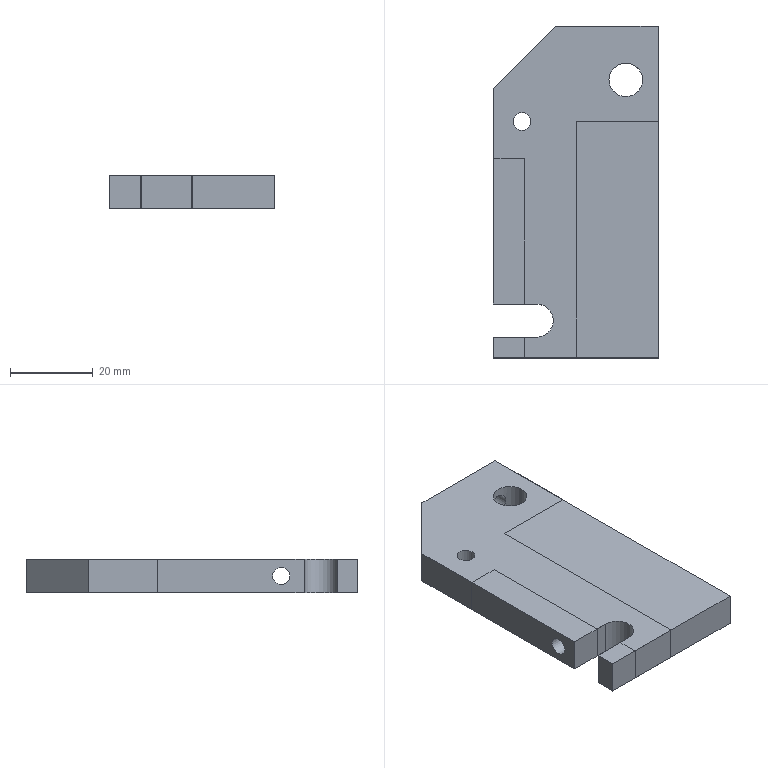NC program | NX | posted with a generic post | part box 40 x 80 x 8 mm
Lines 1 to 594 of 5028:
N10 G17 G21 G94 G90
(FLOOR_FACING_1 , TOOL : D63面刀)
N12 T10 M6
N14 G53
N16 G17 G0 G90 X74.501 Y-4.25 B0. C0. S1600 M3
N18 G43 Z20. H10
N20 Z3.
N22 G94 G1 Z0. F600.
N24 X71.501
N26 X-71.499
N28 X-74.499
N30 Z3.
N32 G0 Z20.
N34 M5
(动态粗 , TOOL : D10-30-D10-75-3T-ROUGH)
N36 T01 M6
N38 G53
N40 G17 G0 G90 X0.648 Y-30.538 B0. C0. S3500 M3
N42 G43 Z20. H1
N44 Z-9.5
N46 G94 G1 X0.649 Y-30.513 Z-9.656 F1500.
N48 X0.651 Y-30.488 Z-9.718
N50 X0.653 Y-30.463 Z-9.763
N52 X0.654 Y-30.438 Z-9.8
N54 X0.656 Y-30.413 Z-9.831
N56 X0.658 Y-30.388 Z-9.857
N58 X0.659 Y-30.363 Z-9.88
N60 X0.661 Y-30.338 Z-9.9
N62 X0.663 Y-30.313 Z-9.918
N64 X0.664 Y-30.288 Z-9.933
N66 X0.666 Y-30.263 Z-9.947
N68 X0.668 Y-30.238 Z-9.958
N70 X0.67 Y-30.213 Z-9.968
N72 X0.671 Y-30.188 Z-9.977
N74 X0.673 Y-30.163 Z-9.984
N76 X0.675 Y-30.139 Z-9.99
N78 X0.676 Y-30.114 Z-9.994
N80 X0.678 Y-30.089 Z-9.997
N82 X0.68 Y-30.064 Z-9.999
N84 X0.681 Y-30.039 Z-10.
N86 X0.78 Y-28.563
N88 G3 X0.004 Y-27.512 R1.01
N90 X-3.302 Y-27.236 R17.164
N92 X-10.4 Y-27.2 R609.799
N94 G1 X-39.92 Y-27.198
N96 G2 X-44.233 Y-24.833 R5.635
N98 X-45.879 Y-20.59 R9.347
N100 X-46.182 Y-15.293 R38.398
N102 G1 X-46.198 Y-8.813
N104 X-46.197 Y20.907
N106 G2 X-43.776 Y25.274 R5.651
N108 X-39.489 Y26.895 R9.477
N110 X-34.169 Y27.185 R40.265
N112 G1 X-27.802 Y27.2
N114 X39.905
N116 G2 X44.289 Y24.764 R5.644
N118 X45.888 Y20.544 R9.455
N120 X46.186 Y14.932 R41.303
N122 G1 X46.2 Y8.407
N124 X46.199 Y-20.904
N126 G2 X43.83 Y-25.24 R5.626
N128 X39.561 Y-26.885 R9.38
N130 X34.421 Y-27.182 R38.069
N132 G1 X28.324 Y-27.2
N134 X1.954 Y-27.199
N136 G3 X-3.101 Y-26.959 R831.893
N138 X-12.695 Y-26.9 R554.852
N140 G1 X-38.21 Y-26.899
N142 G2 X-44.133 Y-23.385 R6.951
N144 X-45.608 Y-18.744 R11.82
N146 X-45.887 Y-12.432 R54.95
N148 G1 X-45.898 Y-7.234
N150 X-45.896 Y19.275
N152 G2 X-42.414 Y25.115 R6.947
N154 X-37.684 Y26.616 R11.837
N156 X-31.259 Y26.889 R57.176
N158 G1 X-25.544 Y26.899
N160 X38.285 Y26.898
N162 G2 X44.128 Y23.399 R6.944
N164 X45.619 Y18.668 R11.881
N166 X45.889 Y12.197 R58.369
N168 G1 X45.9 Y6.437
N170 X45.898 Y-19.284
N172 G2 X42.379 Y-25.139 R6.95
N174 X37.691 Y-26.616 R11.885
N176 X31.626 Y-26.887 R54.523
N178 G1 X25.416 Y-26.899
N180 X-22.049
N182 G3 X-25.671 Y-26.63 R21.33
N184 G1 X-37.165 Y-26.59
N186 G2 X-43.919 Y-22.299 R7.823
N188 X-45.333 Y-17.258 R13.801
N190 X-45.59 Y-10.201 R71.27
N192 G1 X-45.597 Y-4.688
N194 X-45.596 Y17.767
N196 G2 X-45.011 Y20.934 R8.308
N198 G1 X-44.756 Y21.772
N200 G2 X-43.44 Y23.642 R5.968
N202 X-39.677 Y25.692 R9.483
N204 X-34.216 Y26.497 R22.085
N206 X-23.327 Y26.599 R295.884
N208 G1 X37.11 Y26.597
N210 G2 X42.046 Y24.719 R7.838
N212 X43.644 Y23.64 R5.848
N214 X44.76 Y21.969 R5.993
N216 X45.151 Y19.999 R5.998
N218 X45.584 Y11.682 R68.344
N220 G1 X45.599 Y4.752
N222 X45.598 Y-17.799
N224 G2 X45.066 Y-20.865 R9.957
N226 X44.759 Y-21.972 R6.845
N228 X43.642 Y-23.643 R5.993
N230 X40.631 Y-25.41 R8.735
N232 X35.212 Y-26.444 R18.858
N234 X26.237 Y-26.598 R155.192
N236 G1 X-22.028 Y-26.599
N238 G3 X-28.788 Y-26.311 R62.284
N240 G2 X-36.342 Y-26.273 R388.486
N242 X-43.672 Y-21.376 R8.476
N244 X-45.024 Y-16.246 R15.182
N246 X-45.289 Y-8.828 R76.595
N248 G1 X-45.297 Y-2.871
N250 X-45.294 Y16.813
N252 G2 X-45.149 Y18.515 R18.745
N254 X-45.049 Y20.806 R12.569
N256 G1 X-45.01 Y20.935
N258 G3 X-45.149 Y19.801 R7.15
N260 G1 X-45.142 Y-5.273
N262 G3 X-44.999 Y-13.972 R279.37
N264 X-44.147 Y-19.448 R21.649
N266 X-40.731 Y-24.344 R9.341
N268 X-36.017 Y-25.96 R9.628
N270 X-31.048 Y-26.12 R57.065
N272 G2 X-22.033 Y-26.376 R133.369
N274 G3 X-15.103 Y-26.419 R507.848
N276 G1 X26.84 Y-26.417
N278 G3 X35.206 Y-26.244 R128.235
N280 X40.784 Y-25.076 R18.643
N282 G1 X40.828 Y-25.069
N284 G2 X41.53 Y-25.268 R1.004
N286 G1 X41.911 Y-25.557
N288 X43.494 Y-26.762 Z-9.9
N290 X44.343 Y-27.408 F15000.
N292 G2 X43.066 Y-28.945 R-1.
N294 G1 X42.907 Y-28.8
N296 X42.756 Y-28.647
N298 G2 X42.771 Y-27.371 R1.
N300 G1 X43.101 Y-26.981
N302 X43.625 Y-26.37 Z-9.94 F1500.
N304 X44.139 Y-25.751 Z-9.981
N306 X44.236 Y-25.588 Z-9.99
N308 X44.302 Y-25.411 Z-10.
N310 G3 X42.861 Y-24.283 R1.
N312 G2 X41.004 Y-25.051 R5.993
N314 G3 X38.201 Y-25.528 R38.301
N316 G2 X30.647 Y-26.085 R49.65
N318 G1 X21.962 Y-26.118
N320 X-22.05
N322 G3 X-31.227 Y-25.819 R116.087
N324 G2 X-36.099 Y-25.571 R36.261
N326 X-43.332 Y-20.007 R9.13
N328 X-44.582 Y-14.592 R17.257
N330 X-44.822 Y-6.884 R103.267
N332 G3 X-45.05 Y-6.003 R3.921
N334 G1 X-45.149 Y-4.999
N336 X-45.05 Y-6.003
N338 G2 X-44.676 Y-8.251 R6.773
N340 G3 X-44.401 Y-14.345 R126.853
N342 X-43.172 Y-19.671 R17.075
N344 X-36.263 Y-25.201 R9.31
N346 X-31.293 Y-25.624 R27.277
N348 G2 X-22.103 Y-25.903 R200.668
N350 G3 X-15.398 Y-25.938 R596.63
N352 G1 X26.272 Y-25.935
N354 G3 X34.997 Y-25.713 R120.117
N356 X39.228 Y-25.15 R47.983
N358 X40.628 Y-25.088 R8.892
N360 G2 X38.425 Y-25.153 R16.629
N362 X31.947 Y-25.552 R186.605
N364 X20.833 Y-25.638 R443.865
N366 G1 X-22.055 Y-25.637
N368 G3 X-31.429 Y-25.314 R185.596
N370 G2 X-36.227 Y-24.781 R22.044
N372 X-42.871 Y-18.96 R9.656
N374 X-44.105 Y-13.401 R18.485
N376 X-44.404 Y-8.178 R346.915
N378 G3 X-44.757 Y-6.969 R2.18
N380 G1 X-44.835 Y-6.711
N382 G3 X-44.509 Y-7.435 R2.576
N384 G2 X-44.183 Y-9.547 R8.72
N386 G3 X-43.711 Y-14.942 R63.577
N388 X-41.879 Y-20.246 R13.902
N390 X-35.627 Y-24.592 R9.847
N392 X-30.513 Y-25.138 R25.597
N394 G2 X-21.928 Y-25.431 R464.915
N396 G1 X-16.348 Y-25.458
N398 X26.101 Y-25.451
N400 G3 X35.881 Y-25.15 R132.08
N402 G1 X38.536
N404 X35.001
N406 G3 X31.803 Y-25.09 R30.364
N408 G1 X27.001 Y-25.15
N410 X-24.999
N412 G3 X-30.751 Y-24.824 R81.647
N414 G2 X-35.731 Y-24.131 R21.065
N416 X-42.44 Y-17.9 R10.175
N418 X-43.636 Y-12.375 R20.228
N420 G3 X-44.039 Y-8.494 R56.849
N422 X-44.227 Y-7.934 R1.686
N424 X-45.255 Y-7.51 R1.001
N426 X-45.972 Y-8.073 Z-9.953 R1.044
N428 G1 X-46.494 Y-8.978 Z-9.9
N430 X-47.289 Y-10.357 F15000.
N432 G3 X-47.393 Y-11.099 R1.004
N434 G1 X-45.754 Y-17.652
N436 G3 X-44.169 Y-21.243 R11.564
N438 X-41.829 Y-24.123 R18.085
N440 X-40.78 Y-25.115 R14.214
N442 X-38.973 Y-26.255 R8.771
N444 X-36.527 Y-27.13 R12.809
N446 X-34.7 Y-27.481 R16.79
N448 G1 X-29.17 Y-28.216
N450 G3 X-28.633 Y-28.139 R1.014
N452 G1 X-26.927 Y-27.381
N454 X-25.827 Y-26.888 Z-9.961 F1500.
N456 G3 X-25.34 Y-26.301 Z-10. R1.
N458 X-26.005 Y-25.051 R1.
N460 X-28.84 Y-24.65 R12.759
N462 G2 X-33.753 Y-24.185 R43.783
N464 X-39.955 Y-20.891 R10.712
N466 X-42.766 Y-15.247 R12.683
N468 X-43.497 Y-10.396 R39.089
N470 G3 X-43.897 Y-8.363 R7.899
N472 G1 X-44.282 Y-7.86
N474 X-44.536 Y-7.384
N476 G3 X-43.923 Y-8.299 R3.13
N478 G2 X-43.417 Y-10.079 R5.332
N480 G3 X-42.693 Y-14.587 R71.276
N482 X-40.254 Y-20.049 R13.331
N484 X-33.988 Y-23.841 R10.817
N486 X-29.265 Y-24.434 R32.552
N488 G2 X-27.106 Y-24.694 R13.238
N490 G1 X-27.064 Y-24.71
N492 G2 X-26.485 Y-25.473 R1.001
N494 G1 X-26.478 Y-25.73 Z-9.987
N496 X-26.497 Y-25.985 Z-9.974
N498 X-26.598 Y-27.458 Z-9.9
N500 X-26.654 Y-28.281 F15000.
N502 G2 X-28.222 Y-29.034 R1.
N504 G1 X-28.414 Y-28.901
N506 X-28.599 Y-28.758
N508 G2 X-27.986 Y-27.037 R1.
N510 G1 X-27.186 Y-26.986 Z-9.94 F1500.
N512 X-26.388 Y-26.922 Z-9.981
N514 G3 X-26.025 Y-26.797 Z-10. R1.03
N516 X-26.242 Y-24.979 R1.
N518 G2 X-27.456 Y-24.552 R10.429
N520 G3 X-30.655 Y-24.041 R22.096
N522 G2 X-35.467 Y-22.949 R18.562
N524 X-41.568 Y-16.679 R10.962
N526 X-42.779 Y-12.027 R22.305
N528 G3 X-43.431 Y-9. R19.057
N530 X-43.631 Y-8.65 R2.603
N532 X-44.173 Y-8.372 R1.008
N534 G1 X-45.101 Y-8.217
N536 X-47.064 Y-7.89 Z-9.9
N538 X-47.487 Y-7.808 F15000.
N540 G2 X-47.955 Y-7.492 R1.012
N542 G1 X-48.166 Y-7.242
N544 X-48.362 Y-6.98
N546 G2 X-47.615 Y-5.475 R1.
N548 X-46.772 Y-5.78 Z-9.947 R1.046 F1500.
N550 G1 X-45.972 Y-6.478 Z-10.
N552 X-44.065 Y-8.145
N554 G2 X-43.067 Y-9.947 R3.362
N556 X-42.22 Y-13.848 R295.691
N558 G3 X-39.852 Y-19.184 R14.319
N560 X-33.588 Y-23.252 R11.269
N562 X-29.271 Y-24.031 R39.037
N564 G2 X-27.661 Y-24.388 R9.292
N566 G1 X-27.125 Y-24.675
N568 G3 X-29.644 Y-23.765 R7.034
N570 G2 X-33.86 Y-22.776 R34.552
N572 X-41.088 Y-15.927 R11.534
N574 X-42.43 Y-11.307 R30.64
N576 G3 X-43.154 Y-9.148 R8.646
N578 G1 X-43.637 Y-8.645
N580 G2 X-42.637 Y-10.197 R3.12
N582 X-41.612 Y-13.77 R106.237
N584 G3 X-38.954 Y-18.993 R14.448
N586 X-33.059 Y-22.74 R12.062
N588 X-29.155 Y-23.709 R90.995
N590 G2 X-28.061 Y-24.117 R3.935
N592 X-29.24 Y-25.729 R1.
N594 G1 X-29.469 Y-25.58
N596 X-30.144 Y-25.139 Z-9.959
N598 X-30.825 Y-24.707 Z-9.919
N600 X-30.997 Y-24.632 Z-9.909
N602 X-31.18 Y-24.59 Z-9.9
N604 G3 X-31.938 Y-26.355 R1. F15000.
N606 X-31.508 Y-26.661 R1.939
N608 X-30.847 Y-26.713 R1.006
N610 G1 X-29.335 Y-26.312
N612 X-28.172 Y-25.998 Z-9.961 F1500.
N614 G3 X-27.598 Y-25.495 Z-10. R1.
N616 X-27.861 Y-24.281 R1.
N618 X-29.487 Y-23.451 R4.047
N620 G2 X-33.275 Y-22.297 R75.564
N622 X-40.571 Y-15.362 R12.276
N624 X-41.997 Y-11.238 R42.866
N626 G3 X-42.707 Y-9.579 R6.501
N628 G1 X-43.214 Y-9.068
N630 G2 X-42.016 Y-10.864 R3.95
N632 G3 X-40.634 Y-14.655 R152.008
N634 X-36.366 Y-20.323 R13.006
N636 X-31.544 Y-22.62 R16.119
N638 G2 X-28.668 Y-23.636 R20.841
N640 G1 X-28.147 Y-24.046
N642 G3 X-30.235 Y-22.83 R5.855
N644 G2 X-34.11 Y-21.225 R35.126
N646 X-40.074 Y-14.858 R13.248
N648 X-41.588 Y-11.183 R91.093
N650 G3 X-42.132 Y-10.149 R4.733
N652 G1 X-42.689 Y-9.593
N654 G2 X-41.321 Y-11.529 R4.83
N656 G3 X-39.5 Y-15.496 R49.986
N658 X-32.737 Y-21.595 R13.752
N660 G2 X-29.562 Y-22.955 R122.27
N662 X-28.641 Y-23.641 R2.519
N664 G3 X-30.47 Y-22.343 R5.333
N666 G2 X-34.25 Y-20.397 R38.973
N668 X-39.587 Y-14.436 R14.757
N670 G3 X-41.259 Y-11.071 R124.883
N672 X-42.092 Y-10.19 R7.23
N674 G2 X-41.005 Y-11.399 R6.851
N676 X-39.312 Y-14.532 R96.795
N678 G3 X-32.473 Y-21.12 R15.613
N680 G2 X-29.65 Y-22.643 R33.886
N682 G1 X-29.088 Y-23.194
N684 G3 X-31.435 Y-21.402 R8.4
N686 G2 X-35.617 Y-18.541 R23.515
N688 X-39.276 Y-13.816 R18.416
N690 G3 X-40.46 Y-11.822 R22.844
N692 G1 X-41.351 Y-10.931
N694 G2 X-40.042 Y-12.335 R11.058
N696 G3 X-37.924 Y-15.576 R147.018
N698 X-32.466 Y-20.541 R18.138
N700 G2 X-30.435 Y-21.847 R38.887
N702 G1 X-29.751 Y-22.531
N704 G3 X-32.145 Y-20.467 R13.195
N706 G2 X-36.818 Y-16.349 R22.597
N708 X-39.16 Y-13.122 R48.88
N710 G1 X-40.385 Y-11.897
N712 G2 X-38.555 Y-13.817 R22.095
N714 G3 X-35.631 Y-17.321 R34.438
N716 G1 X-33.458 Y-19.494
N718 G2 X-33.179 Y-20.033 R1.009
N720 X-33.749 Y-21.115 Z-9.934 R1.026
N722 G1 X-34.335 Y-21.454 Z-9.9
N724 X-35.205 Y-21.955 F15000.
N726 G3 X-34.582 Y-23.814 R1.
N728 G1 X-32.368 Y-23.454
N730 X-31.181 Y-23.254 Z-9.961 F1500.
N732 G3 X-30.561 Y-22.807 Z-10. R1.
N734 X-30.706 Y-21.576 R1.
N736 X-32.905 Y-19.529 R41.335
N738 G2 X-36.543 Y-15.951 R154.299
N740 G1 X-37.245 Y-15.037
N742 X-39.061 Y-13.221
N744 X-31.44 Y-20.842
N746 G2 X-32.167 Y-22.549 R1.
N748 X-32.656 Y-22.415 Z-9.974 R1.159
N750 G1 X-33.997 Y-21.796 Z-9.9
N752 X-35.628 Y-21.043 F15000.
N754 X-35.78 Y-20.954
N756 X-35.916 Y-20.842
N758 X-46.062 Y-10.697
N760 G2 X-47.848 Y-7.667 R7.038
N762 X-48.35 Y-4.105 R12.901
N764 G1 Y19.884
N766 G2 X-47.742 Y22.858 R7.589
N768 G1 X-47.135 Y24.283
N770 G2 X-45.967 Y24.859 R1.
N772 G1 X-45.762 Y24.807
N774 X-43.835 Y24.313 Z-10. F1500.
N776 X-43.535 Y24.234
N778 X-43.232 Y24.17
N780 G3 X-42.659 Y24.283 R1.01
N782 G2 X-40.802 Y25.051 R5.993
N784 X-33.081 Y26.205 R29.747
N786 X-21.877 Y26.299 R363.029
N788 G1 X37.053
N790 G2 X40.515 Y25.129 R11.382
N792 G1 X40.711 Y25.08
N794 G3 X41.563 Y25.415 R1.001
N796 X41.81 Y25.963 Z-9.969 R1.099
N798 G1 X42.098 Y27.313 Z-9.9
N800 X42.29 Y28.217 F15000.
N802 G2 X42.949 Y28.956 R1.001
N804 G1 X43.149 Y29.023
N806 X43.351 Y29.08
N808 G2 X44.451 Y27.721 R1.
N810 G1 X43.971 Y26.532
N812 X43.413 Y25.161 Z-9.974 F1500.
N814 G2 X43.086 Y24.778 Z-10. R1.007
N816 X42.046 Y24.719 R1.001
N818 G3 X40.517 Y25.115 R5.302
N820 X37.54 Y25.892 R16.316
N822 X32.688 Y26.112 R39.312
N824 G1 X28.143 Y26.119
N826 X-34.847
N828 G2 X-35.324 Y26.24 R1.021
N830 X-35.819 Y26.864 Z-9.959 R1.06
N832 G1 X-36.226 Y27.964 Z-9.9
N834 X-36.532 Y28.791 F15000.
N836 G3 X-38.012 Y29.284 R1.
N838 G1 X-38.6 Y28.904
N840 X-40.452 Y27.59
N842 X-41.535 Y26.816 Z-9.967 F1500.
N844 G3 X-41.875 Y26.268 Z-10. R1.002
N846 X-40.802 Y25.051 R1.
N848 X-37.209 Y25.535 R83.103
N850 G2 X-31.504 Y25.807 R46.5
N852 G1 X-25.249 Y25.819
N854 X35.666 Y25.818
N856 G2 X39.198 Y25.152 R27.238
N858 X40.674 Y25.084 R9.499
N860 G3 X39.04 Y25.157 R12.107
N862 X35.698 Y25.557 R44.815
N864 X27.825 Y25.638 R186.003
N866 G1 X-34.6
N868 G3 X-38.618 Y25.15 R165.75
N870 X-40.067 Y25.124 R14.322
N872 G2 X-37.408 Y25.153 R35.996
N874 X-29.423 Y25.336 R114.742
N876 G1 X-25.913 Y25.338
N878 X35.666
N880 X37.009 Y25.15
N882 X39.169
N884 X-37.511
N886 G2 X-38.205 Y26.871 R1.
N888 X-37.765 Y27.122 Z-9.974 R1.159
N890 G1 X-36.378 Y27.633 Z-9.9
N892 X-34.692 Y28.254 F15000.
N894 X-34.522 Y28.298
N896 X-34.346 Y28.315
N898 X42.761
N900 G2 X46.309 Y26.095 R3.946
N902 G1 X47.389 Y23.876
N904 G2 X47.245 Y22.782 R1.001
N906 G1 X47.16 Y22.684
N908 X45.855 Y21.182 Z-10. F1500.
N910 X45.577 Y20.867
N912 X45.311 Y20.541
N914 G3 X45.151 Y19.999 R1.012
N916 X45.256 Y13.367 R202.115
N918 G2 X45.299 Y3.422 R702.283
N920 G1 X45.298 Y-16.494
N922 G2 X45.151 Y-18.512 R16.383
N924 X45.065 Y-20.874 R15.502
N926 G1 X45.151 Y-20.001
N928 Y17.593
N930 G2 X46.872 Y18.287 R1.
N932 X47.124 Y17.846 Z-9.974 R1.159
N934 G1 X47.634 Y16.46 Z-9.9
N936 X48.255 Y14.774 F15000.
N938 X48.299 Y14.603
N940 X48.316 Y14.428
N942 Y-19.764
N944 G2 X47.282 Y-24.099 R9.496
N946 X45.519 Y-26.311 R7.655
N948 G1 X45.133 Y-26.643
N950 X44.74 Y-26.967
N952 G2 X40.678 Y-28.311 R6.568
N954 G1 X37.717 Y-28.275
N956 G2 X36.912 Y-27.85 R1.001
N958 G1 X36.774 Y-27.655
N960 X35.63 Y-26.027 Z-10. F1500.
N962 X35.416 Y-25.719
N964 X35.19 Y-25.419
N966 G3 X34.552 Y-25.11 R1.005
N968 G2 X33.084 Y-24.92 R65.093
N970 G3 X28.676 Y-24.86 R37.747
N972 G2 X27.06 Y-25.145 R5.456
N974 G3 X28.779 Y-24.833 R5.709
N976 G2 X33.146 Y-24.806 R17.464
N978 G1 X33.189 Y-24.819
N980 G2 X33.676 Y-26.393 R1.1
N982 X32.662 Y-26.923 Z-9.94 R1.135
N984 G1 X31.874 Y-26.941 Z-9.9
N986 X30.065 Y-26.982 F15000.
N988 X29.517 Y-26.996 Z-9.928 F1500.
N990 X28.969 Y-27.001 Z-9.955
N992 G2 X28.189 Y-26.62 Z-10. R1.1
N994 X28.735 Y-24.844 R1.1
N996 X31.422 Y-24.562 R9.406
N998 X32.919 Y-24.691 R5.252
N1000 G1 X32.94 Y-24.7
N1002 G2 X33.421 Y-26.238 R1.1
N1004 X32.413 Y-26.796 Z-9.939 R1.134
N1006 G1 X31.635 Y-26.827 Z-9.9
N1008 X30.275 Y-26.881 F15000.
N1010 X29.72 Y-26.908 Z-9.928 F1500.
N1012 X29.165 Y-26.916 Z-9.956
N1014 G2 X28.411 Y-26.512 Z-10. R1.116
N1016 X28.794 Y-24.828 R1.1
N1018 X30.899 Y-24.451 R6.021
N1020 X32.61 Y-24.547 R5.797
N1022 G3 X34.031 Y-25.053 R5.339
N1024 G2 X32.432 Y-24.468 R6.36
N1026 G3 X29.613 Y-24.438 R5.714
N1028 G1 X28.872 Y-24.791
N1030 G2 X30.105 Y-24.289 R4.975
N1032 X32.238 Y-24.355 R4.462
N1034 G1 X32.319 Y-24.395
N1036 G2 X31.777 Y-26.447 R1.1
N1038 G1 X30.223 Y-26.461
N1040 G2 X29.62 Y-24.435 R1.1
N1042 X32.133 Y-24.275 R3.5
N1044 G1 X32.232 Y-24.329
N1046 G2 X31.701 Y-26.342 R1.094
N1048 G1 X30.315 Y-26.415
N1050 G2 X29.62 Y-24.435 R1.094
N1052 X32.024 Y-24.194 R2.964
N1054 G1 X32.141 Y-24.261
N1056 G2 X31.623 Y-26.246 R1.1
N1058 G1 X30.441 Y-26.382
N1060 G2 X29.675 Y-24.395 R1.1
N1062 X31.927 Y-24.123 R2.593
N1064 G3 X32.543 Y-24.511 R5.845
N1066 G2 X31.839 Y-24.061 R6.584
N1068 G3 X30.05 Y-24.126 R2.165
N1070 G1 X29.74 Y-24.349
N1072 G2 X31.855 Y-24.056 R1.863
N1074 G1 X31.965 Y-24.135
N1076 G3 X30.079 Y-24.105 R1.492
N1078 G2 X31.8 Y-24.016 R1.37
N1080 G3 X30.29 Y-23.954 R1.169
N1082 G2 X31.609 Y-23.88 R1.052
N1084 G3 X30.431 Y-23.855 R1.007
N1086 X30.058 Y-25.068 R1.01
N1088 G1 X30.7 Y-26.673
N1090 X30.709 Y-26.697 Z-9.999
N1092 X30.718 Y-26.72 Z-9.997
N1094 X30.728 Y-26.743 Z-9.994
N1096 X30.737 Y-26.766 Z-9.99
N1098 X30.746 Y-26.79 Z-9.984
N1100 X30.756 Y-26.813 Z-9.977
N1102 X30.765 Y-26.836 Z-9.968
N1104 X30.774 Y-26.859 Z-9.958
N1106 X30.783 Y-26.882 Z-9.947
N1108 X30.793 Y-26.906 Z-9.933
N1110 X30.802 Y-26.929 Z-9.918
N1112 X30.811 Y-26.952 Z-9.9
N1114 X30.821 Y-26.975 Z-9.88
N1116 X30.83 Y-26.998 Z-9.857
N1118 X30.839 Y-27.022 Z-9.831
N1120 X30.848 Y-27.045 Z-9.8
N1122 X30.858 Y-27.068 Z-9.763
N1124 X30.867 Y-27.091 Z-9.718
N1126 X30.876 Y-27.114 Z-9.656
N1128 X30.886 Y-27.138 Z-9.5
N1130 G0 Z20.
N1132 M5
(DRILLING , TOOL : 倒角D10-90度)
N1134 T02 M6
N1136 G53
N1138 G17 G0 G90 X-26.999 Y12. B0. C0. S1200 M3
N1140 G43 Z20. H2
N1142 G94 G81 G99 Z-2.5 F60. R3.
N1144 X-16.999 Y-13.
N1146 G80
N1148 G0 X-16.999 Y-13. Z20.
N1150 M5
(DRILLING_COPY , TOOL : 钻头D4.3-54-83)
N1152 T13 M6
N1154 G53
N1156 G17 G0 G90 X-26.999 Y12. B0. C0. S1600 M3
N1158 G43 Z20. H13
N1160 G94 G83 G99 Z-12. F60. Q2. R3.
N1162 X-16.999 Y-13.
N1164 G80
N1166 G0 X-16.999 Y-13. Z20.
N1168 M5